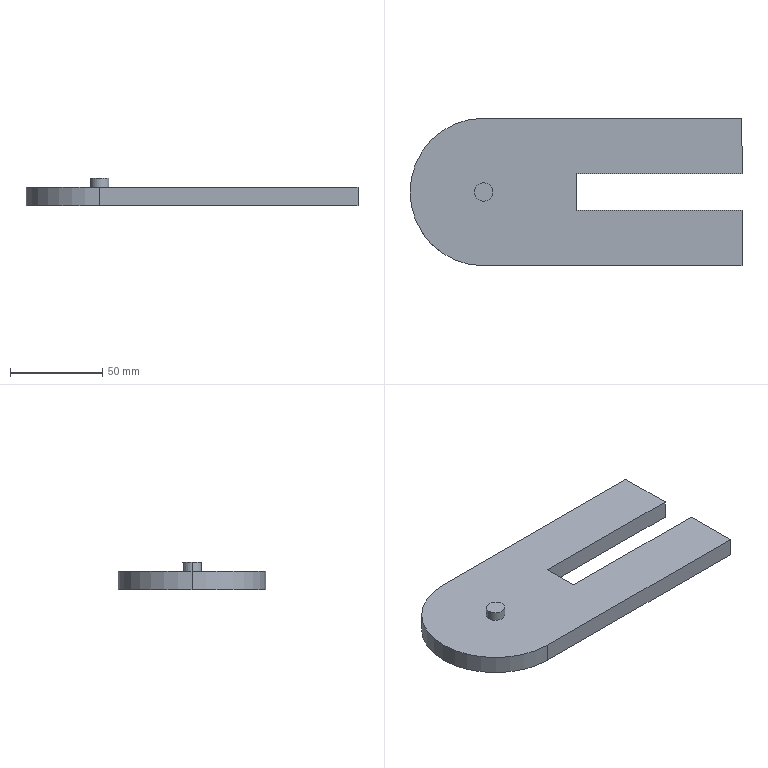Part | SolidWorks | features Boss 1, Extrusion 1 | 1 solid | 14 faces | box 180 x 80 x 15 mm | volume 119525 mm3 | plane 10 | cylinder 4 | commonest cylinder face diameters 10 x2 80 x2
STEP:
#1=CARTESIAN_POINT('',(5.,0.,15.));
#2=VERTEX_POINT('',#1);
#3=CARTESIAN_POINT('',(-5.,0.,15.));
#4=VERTEX_POINT('',#3);
#5=CARTESIAN_POINT('',(0.,0.,15.));
#6=DIRECTION('',(0.,0.,1.));
#7=DIRECTION('',(1.,0.,0.));
#8=AXIS2_PLACEMENT_3D('',#5,#6,#7);
#9=CIRCLE('',#8,5.);
#10=EDGE_CURVE('',#2,#4,#9,.T.);
#11=ORIENTED_EDGE('',*,*,#10,.F.);
#12=CARTESIAN_POINT('',(5.,0.,10.));
#13=VERTEX_POINT('',#12);
#14=CARTESIAN_POINT('',(5.,0.,15.));
#15=DIRECTION('',(0.,0.,-1.));
#16=VECTOR('',#15,1000.);
#17=LINE('',#14,#16);
#18=EDGE_CURVE('',#2,#13,#17,.T.);
#19=ORIENTED_EDGE('',*,*,#18,.T.);
#20=CARTESIAN_POINT('',(-5.,0.,10.));
#21=VERTEX_POINT('',#20);
#22=CARTESIAN_POINT('',(0.,0.,10.));
#23=DIRECTION('',(0.,0.,1.));
#24=DIRECTION('',(1.,0.,0.));
#25=AXIS2_PLACEMENT_3D('',#22,#23,#24);
#26=CIRCLE('',#25,5.);
#27=EDGE_CURVE('',#13,#21,#26,.T.);
#28=ORIENTED_EDGE('',*,*,#27,.T.);
#29=CARTESIAN_POINT('',(-5.,0.,15.));
#30=DIRECTION('',(0.,0.,-1.));
#31=VECTOR('',#30,1000.);
#32=LINE('',#29,#31);
#33=EDGE_CURVE('',#4,#21,#32,.T.);
#34=ORIENTED_EDGE('',*,*,#33,.F.);
#35=EDGE_LOOP('',(#11,#19,#28,#34));
#36=FACE_OUTER_BOUND('',#35,.T.);
#37=CARTESIAN_POINT('',(0.,0.,15.));
#38=DIRECTION('',(0.,0.,-1.));
#39=DIRECTION('',(-1.,0.,0.));
#40=AXIS2_PLACEMENT_3D('',#37,#38,#39);
#41=CYLINDRICAL_SURFACE('',#40,5.);
#42=ADVANCED_FACE('',(#36),#41,.T.);
#43=CARTESIAN_POINT('',(-40.,0.,10.));
#44=VERTEX_POINT('',#43);
#45=CARTESIAN_POINT('',(0.,-40.,10.));
#46=VERTEX_POINT('',#45);
#47=CARTESIAN_POINT('',(0.,0.,10.));
#48=DIRECTION('',(0.,0.,1.));
#49=DIRECTION('',(1.,0.,0.));
#50=AXIS2_PLACEMENT_3D('',#47,#48,#49);
#51=CIRCLE('',#50,40.);
#52=EDGE_CURVE('',#44,#46,#51,.T.);
#53=ORIENTED_EDGE('',*,*,#52,.F.);
#54=CARTESIAN_POINT('',(-40.,0.,0.));
#55=VERTEX_POINT('',#54);
#56=CARTESIAN_POINT('',(-40.,0.,10.));
#57=DIRECTION('',(0.,0.,-1.));
#58=VECTOR('',#57,1000.);
#59=LINE('',#56,#58);
#60=EDGE_CURVE('',#44,#55,#59,.T.);
#61=ORIENTED_EDGE('',*,*,#60,.T.);
#62=CARTESIAN_POINT('',(0.,-40.,0.));
#63=VERTEX_POINT('',#62);
#64=CARTESIAN_POINT('',(0.,0.,0.));
#65=DIRECTION('',(0.,0.,1.));
#66=DIRECTION('',(1.,0.,0.));
#67=AXIS2_PLACEMENT_3D('',#64,#65,#66);
#68=CIRCLE('',#67,40.);
#69=EDGE_CURVE('',#55,#63,#68,.T.);
#70=ORIENTED_EDGE('',*,*,#69,.T.);
#71=CARTESIAN_POINT('',(0.,-40.,10.));
#72=DIRECTION('',(0.,0.,-1.));
#73=VECTOR('',#72,1000.);
#74=LINE('',#71,#73);
#75=EDGE_CURVE('',#46,#63,#74,.T.);
#76=ORIENTED_EDGE('',*,*,#75,.F.);
#77=EDGE_LOOP('',(#53,#61,#70,#76));
#78=FACE_OUTER_BOUND('',#77,.T.);
#79=CARTESIAN_POINT('',(0.,0.,10.));
#80=DIRECTION('',(0.,0.,-1.));
#81=DIRECTION('',(-1.,0.,0.));
#82=AXIS2_PLACEMENT_3D('',#79,#80,#81);
#83=CYLINDRICAL_SURFACE('',#82,40.);
#84=ADVANCED_FACE('',(#78),#83,.T.);
#85=CARTESIAN_POINT('',(0.,40.,10.));
#86=VERTEX_POINT('',#85);
#87=CARTESIAN_POINT('',(0.,0.,10.));
#88=DIRECTION('',(0.,0.,1.));
#89=DIRECTION('',(1.,0.,0.));
#90=AXIS2_PLACEMENT_3D('',#87,#88,#89);
#91=CIRCLE('',#90,40.);
#92=EDGE_CURVE('',#86,#44,#91,.T.);
#93=ORIENTED_EDGE('',*,*,#92,.T.);
#94=ORIENTED_EDGE('',*,*,#52,.T.);
#95=CARTESIAN_POINT('',(140.,-40.,10.));
#96=VERTEX_POINT('',#95);
#97=CARTESIAN_POINT('',(0.,-40.,10.));
#98=DIRECTION('',(1.,0.,0.));
#99=VECTOR('',#98,1000.);
#100=LINE('',#97,#99);
#101=EDGE_CURVE('',#46,#96,#100,.T.);
#102=ORIENTED_EDGE('',*,*,#101,.T.);
#103=CARTESIAN_POINT('',(140.,-10.,10.));
#104=VERTEX_POINT('',#103);
#105=CARTESIAN_POINT('',(140.,-40.,10.));
#106=DIRECTION('',(0.,1.,0.));
#107=VECTOR('',#106,1000.);
#108=LINE('',#105,#107);
#109=EDGE_CURVE('',#96,#104,#108,.T.);
#110=ORIENTED_EDGE('',*,*,#109,.T.);
#111=CARTESIAN_POINT('',(50.,-10.,10.));
#112=VERTEX_POINT('',#111);
#113=CARTESIAN_POINT('',(50.,-10.,10.));
#114=DIRECTION('',(-1.,0.,0.));
#115=VECTOR('',#114,1000.);
#116=LINE('',#113,#115);
#117=EDGE_CURVE('',#104,#112,#116,.T.);
#118=ORIENTED_EDGE('',*,*,#117,.T.);
#119=CARTESIAN_POINT('',(50.,10.,10.));
#120=VERTEX_POINT('',#119);
#121=CARTESIAN_POINT('',(50.,10.,10.));
#122=DIRECTION('',(0.,1.,0.));
#123=VECTOR('',#122,1000.);
#124=LINE('',#121,#123);
#125=EDGE_CURVE('',#112,#120,#124,.T.);
#126=ORIENTED_EDGE('',*,*,#125,.T.);
#127=CARTESIAN_POINT('',(140.,10.,10.));
#128=VERTEX_POINT('',#127);
#129=CARTESIAN_POINT('',(50.,10.,10.));
#130=DIRECTION('',(1.,0.,0.));
#131=VECTOR('',#130,1000.);
#132=LINE('',#129,#131);
#133=EDGE_CURVE('',#120,#128,#132,.T.);
#134=ORIENTED_EDGE('',*,*,#133,.T.);
#135=CARTESIAN_POINT('',(140.,40.,10.));
#136=VERTEX_POINT('',#135);
#137=CARTESIAN_POINT('',(140.,40.,10.));
#138=DIRECTION('',(0.,1.,0.));
#139=VECTOR('',#138,1000.);
#140=LINE('',#137,#139);
#141=EDGE_CURVE('',#128,#136,#140,.T.);
#142=ORIENTED_EDGE('',*,*,#141,.T.);
#143=CARTESIAN_POINT('',(0.,40.,10.));
#144=DIRECTION('',(-1.,0.,0.));
#145=VECTOR('',#144,1000.);
#146=LINE('',#143,#145);
#147=EDGE_CURVE('',#136,#86,#146,.T.);
#148=ORIENTED_EDGE('',*,*,#147,.T.);
#149=EDGE_LOOP('',(#93,#94,#102,#110,#118,#126,#134,#142,#148));
#150=FACE_OUTER_BOUND('',#149,.T.);
#151=CARTESIAN_POINT('',(0.,0.,10.));
#152=DIRECTION('',(0.,0.,1.));
#153=DIRECTION('',(1.,0.,0.));
#154=AXIS2_PLACEMENT_3D('',#151,#152,#153);
#155=CIRCLE('',#154,5.);
#156=EDGE_CURVE('',#21,#13,#155,.T.);
#157=ORIENTED_EDGE('',*,*,#156,.F.);
#158=ORIENTED_EDGE('',*,*,#27,.F.);
#159=EDGE_LOOP('',(#157,#158));
#160=FACE_BOUND('',#159,.T.);
#161=CARTESIAN_POINT('',(0.,0.,10.));
#162=DIRECTION('',(0.,0.,1.));
#163=DIRECTION('',(1.,0.,0.));
#164=AXIS2_PLACEMENT_3D('',#161,#162,#163);
#165=PLANE('',#164);
#166=ADVANCED_FACE('',(#150,#160),#165,.T.);
#167=ORIENTED_EDGE('',*,*,#60,.F.);
#168=ORIENTED_EDGE('',*,*,#92,.F.);
#169=CARTESIAN_POINT('',(0.,40.,0.));
#170=VERTEX_POINT('',#169);
#171=CARTESIAN_POINT('',(0.,40.,10.));
#172=DIRECTION('',(0.,0.,-1.));
#173=VECTOR('',#172,1000.);
#174=LINE('',#171,#173);
#175=EDGE_CURVE('',#86,#170,#174,.T.);
#176=ORIENTED_EDGE('',*,*,#175,.T.);
#177=CARTESIAN_POINT('',(0.,0.,0.));
#178=DIRECTION('',(0.,0.,1.));
#179=DIRECTION('',(1.,0.,0.));
#180=AXIS2_PLACEMENT_3D('',#177,#178,#179);
#181=CIRCLE('',#180,40.);
#182=EDGE_CURVE('',#170,#55,#181,.T.);
#183=ORIENTED_EDGE('',*,*,#182,.T.);
#184=EDGE_LOOP('',(#167,#168,#176,#183));
#185=FACE_OUTER_BOUND('',#184,.T.);
#186=CARTESIAN_POINT('',(0.,0.,10.));
#187=DIRECTION('',(0.,0.,-1.));
#188=DIRECTION('',(-1.,0.,0.));
#189=AXIS2_PLACEMENT_3D('',#186,#187,#188);
#190=CYLINDRICAL_SURFACE('',#189,40.);
#191=ADVANCED_FACE('',(#185),#190,.T.);
#192=CARTESIAN_POINT('',(140.,-40.,0.));
#193=VERTEX_POINT('',#192);
#194=CARTESIAN_POINT('',(0.,-40.,0.));
#195=DIRECTION('',(1.,0.,0.));
#196=VECTOR('',#195,1000.);
#197=LINE('',#194,#196);
#198=EDGE_CURVE('',#63,#193,#197,.T.);
#199=ORIENTED_EDGE('',*,*,#198,.T.);
#200=CARTESIAN_POINT('',(140.,-40.,10.));
#201=DIRECTION('',(0.,0.,-1.));
#202=VECTOR('',#201,1000.);
#203=LINE('',#200,#202);
#204=EDGE_CURVE('',#96,#193,#203,.T.);
#205=ORIENTED_EDGE('',*,*,#204,.F.);
#206=ORIENTED_EDGE('',*,*,#101,.F.);
#207=ORIENTED_EDGE('',*,*,#75,.T.);
#208=EDGE_LOOP('',(#199,#205,#206,#207));
#209=FACE_OUTER_BOUND('',#208,.T.);
#210=CARTESIAN_POINT('',(0.,-40.,10.));
#211=DIRECTION('',(0.,1.,0.));
#212=DIRECTION('',(0.,0.,1.));
#213=AXIS2_PLACEMENT_3D('',#210,#211,#212);
#214=PLANE('',#213);
#215=ADVANCED_FACE('',(#209),#214,.F.);
#216=CARTESIAN_POINT('',(140.,-10.,0.));
#217=VERTEX_POINT('',#216);
#218=CARTESIAN_POINT('',(140.,-40.,0.));
#219=DIRECTION('',(0.,1.,0.));
#220=VECTOR('',#219,1000.);
#221=LINE('',#218,#220);
#222=EDGE_CURVE('',#193,#217,#221,.T.);
#223=ORIENTED_EDGE('',*,*,#222,.T.);
#224=CARTESIAN_POINT('',(140.,-10.,10.));
#225=DIRECTION('',(0.,0.,-1.));
#226=VECTOR('',#225,1000.);
#227=LINE('',#224,#226);
#228=EDGE_CURVE('',#104,#217,#227,.T.);
#229=ORIENTED_EDGE('',*,*,#228,.F.);
#230=ORIENTED_EDGE('',*,*,#109,.F.);
#231=ORIENTED_EDGE('',*,*,#204,.T.);
#232=EDGE_LOOP('',(#223,#229,#230,#231));
#233=FACE_OUTER_BOUND('',#232,.T.);
#234=CARTESIAN_POINT('',(140.,-40.,10.));
#235=DIRECTION('',(-1.,0.,0.));
#236=DIRECTION('',(0.,0.,1.));
#237=AXIS2_PLACEMENT_3D('',#234,#235,#236);
#238=PLANE('',#237);
#239=ADVANCED_FACE('',(#233),#238,.F.);
#240=CARTESIAN_POINT('',(50.,-10.,0.));
#241=VERTEX_POINT('',#240);
#242=CARTESIAN_POINT('',(50.,-10.,0.));
#243=DIRECTION('',(-1.,0.,0.));
#244=VECTOR('',#243,1000.);
#245=LINE('',#242,#244);
#246=EDGE_CURVE('',#217,#241,#245,.T.);
#247=ORIENTED_EDGE('',*,*,#246,.T.);
#248=CARTESIAN_POINT('',(50.,-10.,10.));
#249=DIRECTION('',(0.,0.,-1.));
#250=VECTOR('',#249,1000.);
#251=LINE('',#248,#250);
#252=EDGE_CURVE('',#112,#241,#251,.T.);
#253=ORIENTED_EDGE('',*,*,#252,.F.);
#254=ORIENTED_EDGE('',*,*,#117,.F.);
#255=ORIENTED_EDGE('',*,*,#228,.T.);
#256=EDGE_LOOP('',(#247,#253,#254,#255));
#257=FACE_OUTER_BOUND('',#256,.T.);
#258=CARTESIAN_POINT('',(50.,-10.,10.));
#259=DIRECTION('',(0.,-1.,0.));
#260=DIRECTION('',(1.,0.,0.));
#261=AXIS2_PLACEMENT_3D('',#258,#259,#260);
#262=PLANE('',#261);
#263=ADVANCED_FACE('',(#257),#262,.F.);
#264=CARTESIAN_POINT('',(50.,10.,0.));
#265=VERTEX_POINT('',#264);
#266=CARTESIAN_POINT('',(50.,10.,0.));
#267=DIRECTION('',(0.,1.,0.));
#268=VECTOR('',#267,1000.);
#269=LINE('',#266,#268);
#270=EDGE_CURVE('',#241,#265,#269,.T.);
#271=ORIENTED_EDGE('',*,*,#270,.T.);
#272=CARTESIAN_POINT('',(50.,10.,10.));
#273=DIRECTION('',(0.,0.,-1.));
#274=VECTOR('',#273,1000.);
#275=LINE('',#272,#274);
#276=EDGE_CURVE('',#120,#265,#275,.T.);
#277=ORIENTED_EDGE('',*,*,#276,.F.);
#278=ORIENTED_EDGE('',*,*,#125,.F.);
#279=ORIENTED_EDGE('',*,*,#252,.T.);
#280=EDGE_LOOP('',(#271,#277,#278,#279));
#281=FACE_OUTER_BOUND('',#280,.T.);
#282=CARTESIAN_POINT('',(50.,10.,10.));
#283=DIRECTION('',(-1.,0.,0.));
#284=DIRECTION('',(0.,0.,1.));
#285=AXIS2_PLACEMENT_3D('',#282,#283,#284);
#286=PLANE('',#285);
#287=ADVANCED_FACE('',(#281),#286,.F.);
#288=CARTESIAN_POINT('',(140.,10.,0.));
#289=VERTEX_POINT('',#288);
#290=CARTESIAN_POINT('',(50.,10.,0.));
#291=DIRECTION('',(1.,0.,0.));
#292=VECTOR('',#291,1000.);
#293=LINE('',#290,#292);
#294=EDGE_CURVE('',#265,#289,#293,.T.);
#295=ORIENTED_EDGE('',*,*,#294,.T.);
#296=CARTESIAN_POINT('',(140.,10.,10.));
#297=DIRECTION('',(0.,0.,-1.));
#298=VECTOR('',#297,1000.);
#299=LINE('',#296,#298);
#300=EDGE_CURVE('',#128,#289,#299,.T.);
#301=ORIENTED_EDGE('',*,*,#300,.F.);
#302=ORIENTED_EDGE('',*,*,#133,.F.);
#303=ORIENTED_EDGE('',*,*,#276,.T.);
#304=EDGE_LOOP('',(#295,#301,#302,#303));
#305=FACE_OUTER_BOUND('',#304,.T.);
#306=CARTESIAN_POINT('',(50.,10.,10.));
#307=DIRECTION('',(0.,1.,0.));
#308=DIRECTION('',(-1.,0.,0.));
#309=AXIS2_PLACEMENT_3D('',#306,#307,#308);
#310=PLANE('',#309);
#311=ADVANCED_FACE('',(#305),#310,.F.);
#312=CARTESIAN_POINT('',(140.,40.,0.));
#313=VERTEX_POINT('',#312);
#314=CARTESIAN_POINT('',(140.,40.,0.));
#315=DIRECTION('',(0.,1.,0.));
#316=VECTOR('',#315,1000.);
#317=LINE('',#314,#316);
#318=EDGE_CURVE('',#289,#313,#317,.T.);
#319=ORIENTED_EDGE('',*,*,#318,.T.);
#320=CARTESIAN_POINT('',(140.,40.,10.));
#321=DIRECTION('',(0.,0.,-1.));
#322=VECTOR('',#321,1000.);
#323=LINE('',#320,#322);
#324=EDGE_CURVE('',#136,#313,#323,.T.);
#325=ORIENTED_EDGE('',*,*,#324,.F.);
#326=ORIENTED_EDGE('',*,*,#141,.F.);
#327=ORIENTED_EDGE('',*,*,#300,.T.);
#328=EDGE_LOOP('',(#319,#325,#326,#327));
#329=FACE_OUTER_BOUND('',#328,.T.);
#330=CARTESIAN_POINT('',(140.,40.,10.));
#331=DIRECTION('',(-1.,0.,0.));
#332=DIRECTION('',(0.,-1.,0.));
#333=AXIS2_PLACEMENT_3D('',#330,#331,#332);
#334=PLANE('',#333);
#335=ADVANCED_FACE('',(#329),#334,.F.);
#336=CARTESIAN_POINT('',(0.,40.,0.));
#337=DIRECTION('',(-1.,0.,0.));
#338=VECTOR('',#337,1000.);
#339=LINE('',#336,#338);
#340=EDGE_CURVE('',#313,#170,#339,.T.);
#341=ORIENTED_EDGE('',*,*,#340,.T.);
#342=ORIENTED_EDGE('',*,*,#175,.F.);
#343=ORIENTED_EDGE('',*,*,#147,.F.);
#344=ORIENTED_EDGE('',*,*,#324,.T.);
#345=EDGE_LOOP('',(#341,#342,#343,#344));
#346=FACE_OUTER_BOUND('',#345,.T.);
#347=CARTESIAN_POINT('',(0.,40.,10.));
#348=DIRECTION('',(0.,-1.,0.));
#349=DIRECTION('',(0.,0.,-1.));
#350=AXIS2_PLACEMENT_3D('',#347,#348,#349);
#351=PLANE('',#350);
#352=ADVANCED_FACE('',(#346),#351,.F.);
#353=ORIENTED_EDGE('',*,*,#182,.F.);
#354=ORIENTED_EDGE('',*,*,#340,.F.);
#355=ORIENTED_EDGE('',*,*,#318,.F.);
#356=ORIENTED_EDGE('',*,*,#294,.F.);
#357=ORIENTED_EDGE('',*,*,#270,.F.);
#358=ORIENTED_EDGE('',*,*,#246,.F.);
#359=ORIENTED_EDGE('',*,*,#222,.F.);
#360=ORIENTED_EDGE('',*,*,#198,.F.);
#361=ORIENTED_EDGE('',*,*,#69,.F.);
#362=EDGE_LOOP('',(#353,#354,#355,#356,#357,#358,#359,#360,#361));
#363=FACE_OUTER_BOUND('',#362,.T.);
#364=CARTESIAN_POINT('',(0.,0.,0.));
#365=DIRECTION('',(0.,0.,1.));
#366=DIRECTION('',(1.,0.,0.));
#367=AXIS2_PLACEMENT_3D('',#364,#365,#366);
#368=PLANE('',#367);
#369=ADVANCED_FACE('',(#363),#368,.F.);
#370=ORIENTED_EDGE('',*,*,#18,.F.);
#371=CARTESIAN_POINT('',(0.,0.,15.));
#372=DIRECTION('',(0.,0.,1.));
#373=DIRECTION('',(1.,0.,0.));
#374=AXIS2_PLACEMENT_3D('',#371,#372,#373);
#375=CIRCLE('',#374,5.);
#376=EDGE_CURVE('',#4,#2,#375,.T.);
#377=ORIENTED_EDGE('',*,*,#376,.F.);
#378=ORIENTED_EDGE('',*,*,#33,.T.);
#379=ORIENTED_EDGE('',*,*,#156,.T.);
#380=EDGE_LOOP('',(#370,#377,#378,#379));
#381=FACE_OUTER_BOUND('',#380,.T.);
#382=CARTESIAN_POINT('',(0.,0.,15.));
#383=DIRECTION('',(0.,0.,-1.));
#384=DIRECTION('',(-1.,0.,0.));
#385=AXIS2_PLACEMENT_3D('',#382,#383,#384);
#386=CYLINDRICAL_SURFACE('',#385,5.);
#387=ADVANCED_FACE('',(#381),#386,.T.);
#388=ORIENTED_EDGE('',*,*,#376,.T.);
#389=ORIENTED_EDGE('',*,*,#10,.T.);
#390=EDGE_LOOP('',(#388,#389));
#391=FACE_OUTER_BOUND('',#390,.T.);
#392=CARTESIAN_POINT('',(0.,0.,15.));
#393=DIRECTION('',(0.,0.,1.));
#394=DIRECTION('',(1.,0.,0.));
#395=AXIS2_PLACEMENT_3D('',#392,#393,#394);
#396=PLANE('',#395);
#397=ADVANCED_FACE('',(#391),#396,.T.);
#398=CLOSED_SHELL('',(#42,#84,#166,#191,#215,#239,#263,#287,#311,#335,#352,#369,#387,#397));
#399=MANIFOLD_SOLID_BREP('',#398);
#400=CARTESIAN_POINT('',(0.,0.,0.));
#401=DIRECTION('',(0.,0.,1.));
#402=DIRECTION('',(1.,0.,0.));
#403=AXIS2_PLACEMENT_3D('',#400,#401,#402);
#404=(LENGTH_UNIT()NAMED_UNIT(*)SI_UNIT(.MILLI.,.METRE.));
#405=UNCERTAINTY_MEASURE_WITH_UNIT(LENGTH_MEASURE(0.00001),#404,'','');
#406=(NAMED_UNIT(*)PLANE_ANGLE_UNIT()SI_UNIT($,.RADIAN.));
#407=(NAMED_UNIT(*)SI_UNIT($,.STERADIAN.)SOLID_ANGLE_UNIT());
#408=(GEOMETRIC_REPRESENTATION_CONTEXT(3)GLOBAL_UNCERTAINTY_ASSIGNED_CONTEXT((#405))GLOBAL_UNIT_ASSIGNED_CONTEXT((#404,#406,#407))REPRESENTATION_CONTEXT('',''));
#409=ADVANCED_BREP_SHAPE_REPRESENTATION('',(#399,#403),#408);